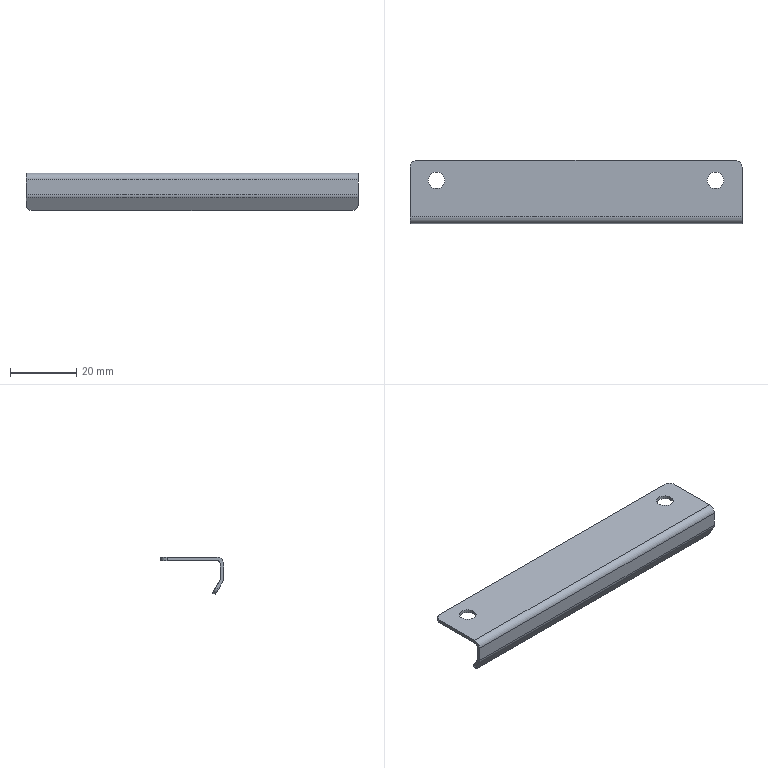Part | NX | features BREP 1 | 1 solid | 22 faces | box 100 x 19 x 11.33 mm | volume 2864 mm3 | cylinder 12 | plane 10 | commonest cylinder face diameters 4 x6 5 x4 2 x2
STEP:
#1=CARTESIAN_POINT('',(-39.5,3.5,1.));
#2=VERTEX_POINT('',#1);
#3=CARTESIAN_POINT('',(-44.5,3.5,1.));
#4=VERTEX_POINT('',#3);
#5=CARTESIAN_POINT('',(-42.,3.5,1.));
#6=DIRECTION('',(0.,0.,-1.));
#7=DIRECTION('',(-1.,0.,0.));
#8=AXIS2_PLACEMENT_3D('',#5,#6,#7);
#9=CIRCLE('',#8,2.5);
#10=EDGE_CURVE('',#2,#4,#9,.T.);
#11=ORIENTED_EDGE('',*,*,#10,.F.);
#12=CARTESIAN_POINT('',(-39.5,3.5,0.));
#13=VERTEX_POINT('',#12);
#14=CARTESIAN_POINT('',(-39.5,3.5,1.));
#15=DIRECTION('',(0.,0.,-1.));
#16=VECTOR('',#15,1000.);
#17=LINE('',#14,#16);
#18=EDGE_CURVE('',#2,#13,#17,.T.);
#19=ORIENTED_EDGE('',*,*,#18,.T.);
#20=CARTESIAN_POINT('',(-44.5,3.5,0.));
#21=VERTEX_POINT('',#20);
#22=CARTESIAN_POINT('',(-42.,3.5,0.));
#23=DIRECTION('',(0.,0.,-1.));
#24=DIRECTION('',(-1.,0.,0.));
#25=AXIS2_PLACEMENT_3D('',#22,#23,#24);
#26=CIRCLE('',#25,2.5);
#27=EDGE_CURVE('',#13,#21,#26,.T.);
#28=ORIENTED_EDGE('',*,*,#27,.T.);
#29=CARTESIAN_POINT('',(-44.5,3.5,1.));
#30=DIRECTION('',(0.,0.,-1.));
#31=VECTOR('',#30,1000.);
#32=LINE('',#29,#31);
#33=EDGE_CURVE('',#4,#21,#32,.T.);
#34=ORIENTED_EDGE('',*,*,#33,.F.);
#35=EDGE_LOOP('',(#11,#19,#28,#34));
#36=FACE_BOUND('',#35,.T.);
#37=CARTESIAN_POINT('',(-42.,3.5,1.));
#38=DIRECTION('',(0.,0.,-1.));
#39=DIRECTION('',(-1.,0.,0.));
#40=AXIS2_PLACEMENT_3D('',#37,#38,#39);
#41=CYLINDRICAL_SURFACE('',#40,2.5);
#42=ADVANCED_FACE('',(#36),#41,.F.);
#43=CARTESIAN_POINT('',(44.5,3.5,1.));
#44=VERTEX_POINT('',#43);
#45=CARTESIAN_POINT('',(39.5,3.5,1.));
#46=VERTEX_POINT('',#45);
#47=CARTESIAN_POINT('',(42.,3.5,1.));
#48=DIRECTION('',(0.,0.,-1.));
#49=DIRECTION('',(-1.,0.,0.));
#50=AXIS2_PLACEMENT_3D('',#47,#48,#49);
#51=CIRCLE('',#50,2.5);
#52=EDGE_CURVE('',#44,#46,#51,.T.);
#53=ORIENTED_EDGE('',*,*,#52,.F.);
#54=CARTESIAN_POINT('',(44.5,3.5,0.));
#55=VERTEX_POINT('',#54);
#56=CARTESIAN_POINT('',(44.5,3.5,1.));
#57=DIRECTION('',(0.,0.,-1.));
#58=VECTOR('',#57,1000.);
#59=LINE('',#56,#58);
#60=EDGE_CURVE('',#44,#55,#59,.T.);
#61=ORIENTED_EDGE('',*,*,#60,.T.);
#62=CARTESIAN_POINT('',(39.5,3.5,0.));
#63=VERTEX_POINT('',#62);
#64=CARTESIAN_POINT('',(42.,3.5,0.));
#65=DIRECTION('',(0.,0.,-1.));
#66=DIRECTION('',(-1.,0.,0.));
#67=AXIS2_PLACEMENT_3D('',#64,#65,#66);
#68=CIRCLE('',#67,2.5);
#69=EDGE_CURVE('',#55,#63,#68,.T.);
#70=ORIENTED_EDGE('',*,*,#69,.T.);
#71=CARTESIAN_POINT('',(39.5,3.5,1.));
#72=DIRECTION('',(0.,0.,-1.));
#73=VECTOR('',#72,1000.);
#74=LINE('',#71,#73);
#75=EDGE_CURVE('',#46,#63,#74,.T.);
#76=ORIENTED_EDGE('',*,*,#75,.F.);
#77=EDGE_LOOP('',(#53,#61,#70,#76));
#78=FACE_BOUND('',#77,.T.);
#79=CARTESIAN_POINT('',(42.,3.5,1.));
#80=DIRECTION('',(0.,0.,-1.));
#81=DIRECTION('',(-1.,0.,0.));
#82=AXIS2_PLACEMENT_3D('',#79,#80,#81);
#83=CYLINDRICAL_SURFACE('',#82,2.5);
#84=ADVANCED_FACE('',(#78),#83,.F.);
#85=CARTESIAN_POINT('',(50.,-9.232,-6.464));
#86=VERTEX_POINT('',#85);
#87=CARTESIAN_POINT('',(50.,-8.,-8.598));
#88=VERTEX_POINT('',#87);
#89=CARTESIAN_POINT('',(50.,-9.5,-6.));
#90=DIRECTION('',(0.,0.5,-0.866));
#91=VECTOR('',#90,1000.);
#92=LINE('',#89,#91);
#93=EDGE_CURVE('',#86,#88,#92,.T.);
#94=ORIENTED_EDGE('',*,*,#93,.T.);
#95=CARTESIAN_POINT('',(50.,-7.134,-8.098));
#96=VERTEX_POINT('',#95);
#97=CARTESIAN_POINT('',(50.,-7.134,-8.098));
#98=DIRECTION('',(0.,0.866,0.5));
#99=VECTOR('',#98,1000.);
#100=LINE('',#97,#99);
#101=EDGE_CURVE('',#88,#96,#100,.T.);
#102=ORIENTED_EDGE('',*,*,#101,.T.);
#103=CARTESIAN_POINT('',(50.,-8.366,-5.964));
#104=VERTEX_POINT('',#103);
#105=CARTESIAN_POINT('',(50.,-8.634,-5.5));
#106=DIRECTION('',(0.,-0.5,0.866));
#107=VECTOR('',#106,1000.);
#108=LINE('',#105,#107);
#109=EDGE_CURVE('',#96,#104,#108,.T.);
#110=ORIENTED_EDGE('',*,*,#109,.T.);
#111=CARTESIAN_POINT('',(50.,-8.5,-5.464));
#112=VERTEX_POINT('',#111);
#113=CARTESIAN_POINT('',(50.,-7.5,-5.464));
#114=DIRECTION('',(-1.,0.,0.));
#115=DIRECTION('',(0.,0.,1.));
#116=AXIS2_PLACEMENT_3D('',#113,#114,#115);
#117=CIRCLE('',#116,1.);
#118=EDGE_CURVE('',#104,#112,#117,.T.);
#119=ORIENTED_EDGE('',*,*,#118,.T.);
#120=CARTESIAN_POINT('',(50.,-8.5,-1.));
#121=VERTEX_POINT('',#120);
#122=CARTESIAN_POINT('',(50.,-8.5,-6.));
#123=DIRECTION('',(0.,0.,1.));
#124=VECTOR('',#123,1000.);
#125=LINE('',#122,#124);
#126=EDGE_CURVE('',#112,#121,#125,.T.);
#127=ORIENTED_EDGE('',*,*,#126,.T.);
#128=CARTESIAN_POINT('',(50.,-7.5,0.));
#129=VERTEX_POINT('',#128);
#130=CARTESIAN_POINT('',(50.,-7.5,-1.));
#131=DIRECTION('',(-1.,0.,0.));
#132=DIRECTION('',(0.,0.,1.));
#133=AXIS2_PLACEMENT_3D('',#130,#131,#132);
#134=CIRCLE('',#133,1.);
#135=EDGE_CURVE('',#121,#129,#134,.T.);
#136=ORIENTED_EDGE('',*,*,#135,.T.);
#137=CARTESIAN_POINT('',(50.,7.5,0.));
#138=VERTEX_POINT('',#137);
#139=CARTESIAN_POINT('',(50.,-9.5,0.));
#140=DIRECTION('',(0.,1.,0.));
#141=VECTOR('',#140,1000.);
#142=LINE('',#139,#141);
#143=EDGE_CURVE('',#129,#138,#142,.T.);
#144=ORIENTED_EDGE('',*,*,#143,.T.);
#145=CARTESIAN_POINT('',(50.,7.5,1.));
#146=VERTEX_POINT('',#145);
#147=CARTESIAN_POINT('',(50.,7.5,1.));
#148=DIRECTION('',(0.,0.,1.));
#149=VECTOR('',#148,1000.);
#150=LINE('',#147,#149);
#151=EDGE_CURVE('',#138,#146,#150,.T.);
#152=ORIENTED_EDGE('',*,*,#151,.T.);
#153=CARTESIAN_POINT('',(50.,-7.5,1.));
#154=VERTEX_POINT('',#153);
#155=CARTESIAN_POINT('',(50.,-9.5,1.));
#156=DIRECTION('',(0.,1.,0.));
#157=VECTOR('',#156,1000.);
#158=LINE('',#155,#157);
#159=EDGE_CURVE('',#154,#146,#158,.T.);
#160=ORIENTED_EDGE('',*,*,#159,.F.);
#161=CARTESIAN_POINT('',(50.,-9.5,-1.));
#162=VERTEX_POINT('',#161);
#163=CARTESIAN_POINT('',(50.,-7.5,-1.));
#164=DIRECTION('',(1.,0.,0.));
#165=DIRECTION('',(0.,0.,1.));
#166=AXIS2_PLACEMENT_3D('',#163,#164,#165);
#167=CIRCLE('',#166,2.);
#168=EDGE_CURVE('',#154,#162,#167,.T.);
#169=ORIENTED_EDGE('',*,*,#168,.T.);
#170=CARTESIAN_POINT('',(50.,-9.5,-5.464));
#171=VERTEX_POINT('',#170);
#172=CARTESIAN_POINT('',(50.,-9.5,1.));
#173=DIRECTION('',(0.,0.,-1.));
#174=VECTOR('',#173,1000.);
#175=LINE('',#172,#174);
#176=EDGE_CURVE('',#162,#171,#175,.T.);
#177=ORIENTED_EDGE('',*,*,#176,.T.);
#178=CARTESIAN_POINT('',(50.,-7.5,-5.464));
#179=DIRECTION('',(1.,0.,0.));
#180=DIRECTION('',(0.,0.,1.));
#181=AXIS2_PLACEMENT_3D('',#178,#179,#180);
#182=CIRCLE('',#181,2.);
#183=EDGE_CURVE('',#171,#86,#182,.T.);
#184=ORIENTED_EDGE('',*,*,#183,.T.);
#185=EDGE_LOOP('',(#94,#102,#110,#119,#127,#136,#144,#152,#160,#169,#177,#184));
#186=FACE_BOUND('',#185,.T.);
#187=CARTESIAN_POINT('',(50.,-9.5,1.));
#188=DIRECTION('',(-1.,0.,0.));
#189=DIRECTION('',(0.,0.,1.));
#190=AXIS2_PLACEMENT_3D('',#187,#188,#189);
#191=PLANE('',#190);
#192=ADVANCED_FACE('',(#186),#191,.F.);
#193=CARTESIAN_POINT('',(48.,9.5,1.));
#194=VERTEX_POINT('',#193);
#195=CARTESIAN_POINT('',(-48.,9.5,1.));
#196=VERTEX_POINT('',#195);
#197=CARTESIAN_POINT('',(-50.,9.5,1.));
#198=DIRECTION('',(-1.,0.,0.));
#199=VECTOR('',#198,1000.);
#200=LINE('',#197,#199);
#201=EDGE_CURVE('',#194,#196,#200,.T.);
#202=ORIENTED_EDGE('',*,*,#201,.F.);
#203=CARTESIAN_POINT('',(48.,9.5,0.));
#204=VERTEX_POINT('',#203);
#205=CARTESIAN_POINT('',(48.,9.5,1.));
#206=DIRECTION('',(0.,0.,-1.));
#207=VECTOR('',#206,1000.);
#208=LINE('',#205,#207);
#209=EDGE_CURVE('',#194,#204,#208,.T.);
#210=ORIENTED_EDGE('',*,*,#209,.T.);
#211=CARTESIAN_POINT('',(-48.,9.5,0.));
#212=VERTEX_POINT('',#211);
#213=CARTESIAN_POINT('',(-50.,9.5,0.));
#214=DIRECTION('',(-1.,0.,0.));
#215=VECTOR('',#214,1000.);
#216=LINE('',#213,#215);
#217=EDGE_CURVE('',#204,#212,#216,.T.);
#218=ORIENTED_EDGE('',*,*,#217,.T.);
#219=CARTESIAN_POINT('',(-48.,9.5,1.));
#220=DIRECTION('',(0.,0.,1.));
#221=VECTOR('',#220,1000.);
#222=LINE('',#219,#221);
#223=EDGE_CURVE('',#212,#196,#222,.T.);
#224=ORIENTED_EDGE('',*,*,#223,.T.);
#225=EDGE_LOOP('',(#202,#210,#218,#224));
#226=FACE_BOUND('',#225,.T.);
#227=CARTESIAN_POINT('',(-50.,9.5,1.));
#228=DIRECTION('',(0.,-1.,0.));
#229=DIRECTION('',(0.,0.,-1.));
#230=AXIS2_PLACEMENT_3D('',#227,#228,#229);
#231=PLANE('',#230);
#232=ADVANCED_FACE('',(#226),#231,.F.);
#233=CARTESIAN_POINT('',(-50.,-8.366,-5.964));
#234=VERTEX_POINT('',#233);
#235=CARTESIAN_POINT('',(-50.,-7.134,-8.098));
#236=VERTEX_POINT('',#235);
#237=CARTESIAN_POINT('',(-50.,-8.634,-5.5));
#238=DIRECTION('',(0.,0.5,-0.866));
#239=VECTOR('',#238,1000.);
#240=LINE('',#237,#239);
#241=EDGE_CURVE('',#234,#236,#240,.T.);
#242=ORIENTED_EDGE('',*,*,#241,.T.);
#243=CARTESIAN_POINT('',(-50.,-8.,-8.598));
#244=VERTEX_POINT('',#243);
#245=CARTESIAN_POINT('',(-50.,-8.,-8.598));
#246=DIRECTION('',(0.,-0.866,-0.5));
#247=VECTOR('',#246,1000.);
#248=LINE('',#245,#247);
#249=EDGE_CURVE('',#236,#244,#248,.T.);
#250=ORIENTED_EDGE('',*,*,#249,.T.);
#251=CARTESIAN_POINT('',(-50.,-9.232,-6.464));
#252=VERTEX_POINT('',#251);
#253=CARTESIAN_POINT('',(-50.,-9.5,-6.));
#254=DIRECTION('',(0.,-0.5,0.866));
#255=VECTOR('',#254,1000.);
#256=LINE('',#253,#255);
#257=EDGE_CURVE('',#244,#252,#256,.T.);
#258=ORIENTED_EDGE('',*,*,#257,.T.);
#259=CARTESIAN_POINT('',(-50.,-9.5,-5.464));
#260=VERTEX_POINT('',#259);
#261=CARTESIAN_POINT('',(-50.,-7.5,-5.464));
#262=DIRECTION('',(-1.,0.,0.));
#263=DIRECTION('',(0.,0.,-1.));
#264=AXIS2_PLACEMENT_3D('',#261,#262,#263);
#265=CIRCLE('',#264,2.);
#266=EDGE_CURVE('',#252,#260,#265,.T.);
#267=ORIENTED_EDGE('',*,*,#266,.T.);
#268=CARTESIAN_POINT('',(-50.,-9.5,-1.));
#269=VERTEX_POINT('',#268);
#270=CARTESIAN_POINT('',(-50.,-9.5,1.));
#271=DIRECTION('',(0.,0.,-1.));
#272=VECTOR('',#271,1000.);
#273=LINE('',#270,#272);
#274=EDGE_CURVE('',#269,#260,#273,.T.);
#275=ORIENTED_EDGE('',*,*,#274,.F.);
#276=CARTESIAN_POINT('',(-50.,-7.5,1.));
#277=VERTEX_POINT('',#276);
#278=CARTESIAN_POINT('',(-50.,-7.5,-1.));
#279=DIRECTION('',(-1.,0.,0.));
#280=DIRECTION('',(0.,0.,-1.));
#281=AXIS2_PLACEMENT_3D('',#278,#279,#280);
#282=CIRCLE('',#281,2.);
#283=EDGE_CURVE('',#269,#277,#282,.T.);
#284=ORIENTED_EDGE('',*,*,#283,.T.);
#285=CARTESIAN_POINT('',(-50.,7.5,1.));
#286=VERTEX_POINT('',#285);
#287=CARTESIAN_POINT('',(-50.,-9.5,1.));
#288=DIRECTION('',(0.,-1.,0.));
#289=VECTOR('',#288,1000.);
#290=LINE('',#287,#289);
#291=EDGE_CURVE('',#286,#277,#290,.T.);
#292=ORIENTED_EDGE('',*,*,#291,.F.);
#293=CARTESIAN_POINT('',(-50.,7.5,0.));
#294=VERTEX_POINT('',#293);
#295=CARTESIAN_POINT('',(-50.,7.5,1.));
#296=DIRECTION('',(0.,0.,-1.));
#297=VECTOR('',#296,1000.);
#298=LINE('',#295,#297);
#299=EDGE_CURVE('',#286,#294,#298,.T.);
#300=ORIENTED_EDGE('',*,*,#299,.T.);
#301=CARTESIAN_POINT('',(-50.,-7.5,0.));
#302=VERTEX_POINT('',#301);
#303=CARTESIAN_POINT('',(-50.,-9.5,0.));
#304=DIRECTION('',(0.,-1.,0.));
#305=VECTOR('',#304,1000.);
#306=LINE('',#303,#305);
#307=EDGE_CURVE('',#294,#302,#306,.T.);
#308=ORIENTED_EDGE('',*,*,#307,.T.);
#309=CARTESIAN_POINT('',(-50.,-8.5,-1.));
#310=VERTEX_POINT('',#309);
#311=CARTESIAN_POINT('',(-50.,-7.5,-1.));
#312=DIRECTION('',(1.,0.,0.));
#313=DIRECTION('',(0.,0.,-1.));
#314=AXIS2_PLACEMENT_3D('',#311,#312,#313);
#315=CIRCLE('',#314,1.);
#316=EDGE_CURVE('',#302,#310,#315,.T.);
#317=ORIENTED_EDGE('',*,*,#316,.T.);
#318=CARTESIAN_POINT('',(-50.,-8.5,-5.464));
#319=VERTEX_POINT('',#318);
#320=CARTESIAN_POINT('',(-50.,-8.5,-6.));
#321=DIRECTION('',(0.,0.,1.));
#322=VECTOR('',#321,1000.);
#323=LINE('',#320,#322);
#324=EDGE_CURVE('',#319,#310,#323,.T.);
#325=ORIENTED_EDGE('',*,*,#324,.F.);
#326=CARTESIAN_POINT('',(-50.,-7.5,-5.464));
#327=DIRECTION('',(1.,0.,0.));
#328=DIRECTION('',(0.,0.,-1.));
#329=AXIS2_PLACEMENT_3D('',#326,#327,#328);
#330=CIRCLE('',#329,1.);
#331=EDGE_CURVE('',#319,#234,#330,.T.);
#332=ORIENTED_EDGE('',*,*,#331,.T.);
#333=EDGE_LOOP('',(#242,#250,#258,#267,#275,#284,#292,#300,#308,#317,#325,#332));
#334=FACE_BOUND('',#333,.T.);
#335=CARTESIAN_POINT('',(-50.,-9.5,1.));
#336=DIRECTION('',(1.,0.,0.));
#337=DIRECTION('',(0.,1.,0.));
#338=AXIS2_PLACEMENT_3D('',#335,#336,#337);
#339=PLANE('',#338);
#340=ADVANCED_FACE('',(#334),#339,.F.);
#341=ORIENTED_EDGE('',*,*,#274,.T.);
#342=CARTESIAN_POINT('',(50.,-9.5,-5.464));
#343=DIRECTION('',(1.,0.,0.));
#344=VECTOR('',#343,1000.);
#345=LINE('',#342,#344);
#346=EDGE_CURVE('',#260,#171,#345,.T.);
#347=ORIENTED_EDGE('',*,*,#346,.T.);
#348=ORIENTED_EDGE('',*,*,#176,.F.);
#349=CARTESIAN_POINT('',(-50.,-9.5,-1.));
#350=DIRECTION('',(-1.,0.,0.));
#351=VECTOR('',#350,1000.);
#352=LINE('',#349,#351);
#353=EDGE_CURVE('',#162,#269,#352,.T.);
#354=ORIENTED_EDGE('',*,*,#353,.T.);
#355=EDGE_LOOP('',(#341,#347,#348,#354));
#356=FACE_BOUND('',#355,.T.);
#357=CARTESIAN_POINT('',(-50.,-9.5,1.));
#358=DIRECTION('',(0.,1.,0.));
#359=DIRECTION('',(1.,0.,0.));
#360=AXIS2_PLACEMENT_3D('',#357,#358,#359);
#361=PLANE('',#360);
#362=ADVANCED_FACE('',(#356),#361,.F.);
#363=ORIENTED_EDGE('',*,*,#159,.T.);
#364=CARTESIAN_POINT('',(48.,7.5,1.));
#365=DIRECTION('',(0.,0.,1.));
#366=DIRECTION('',(-1.,0.,0.));
#367=AXIS2_PLACEMENT_3D('',#364,#365,#366);
#368=CIRCLE('',#367,2.);
#369=EDGE_CURVE('',#146,#194,#368,.T.);
#370=ORIENTED_EDGE('',*,*,#369,.T.);
#371=ORIENTED_EDGE('',*,*,#201,.T.);
#372=CARTESIAN_POINT('',(-48.,7.5,1.));
#373=DIRECTION('',(0.,0.,1.));
#374=DIRECTION('',(-1.,0.,0.));
#375=AXIS2_PLACEMENT_3D('',#372,#373,#374);
#376=CIRCLE('',#375,2.);
#377=EDGE_CURVE('',#196,#286,#376,.T.);
#378=ORIENTED_EDGE('',*,*,#377,.T.);
#379=ORIENTED_EDGE('',*,*,#291,.T.);
#380=CARTESIAN_POINT('',(0.,-7.5,1.));
#381=DIRECTION('',(1.,0.,0.));
#382=VECTOR('',#381,1000.);
#383=LINE('',#380,#382);
#384=EDGE_CURVE('',#277,#154,#383,.T.);
#385=ORIENTED_EDGE('',*,*,#384,.T.);
#386=EDGE_LOOP('',(#363,#370,#371,#378,#379,#385));
#387=FACE_BOUND('',#386,.T.);
#388=CARTESIAN_POINT('',(-42.,3.5,1.));
#389=DIRECTION('',(0.,0.,-1.));
#390=DIRECTION('',(-1.,0.,0.));
#391=AXIS2_PLACEMENT_3D('',#388,#389,#390);
#392=CIRCLE('',#391,2.5);
#393=EDGE_CURVE('',#4,#2,#392,.T.);
#394=ORIENTED_EDGE('',*,*,#393,.T.);
#395=ORIENTED_EDGE('',*,*,#10,.T.);
#396=EDGE_LOOP('',(#394,#395));
#397=FACE_BOUND('',#396,.T.);
#398=CARTESIAN_POINT('',(42.,3.5,1.));
#399=DIRECTION('',(0.,0.,-1.));
#400=DIRECTION('',(-1.,0.,0.));
#401=AXIS2_PLACEMENT_3D('',#398,#399,#400);
#402=CIRCLE('',#401,2.5);
#403=EDGE_CURVE('',#46,#44,#402,.T.);
#404=ORIENTED_EDGE('',*,*,#403,.T.);
#405=ORIENTED_EDGE('',*,*,#52,.T.);
#406=EDGE_LOOP('',(#404,#405));
#407=FACE_BOUND('',#406,.T.);
#408=CARTESIAN_POINT('',(0.,0.,1.));
#409=DIRECTION('',(0.,0.,-1.));
#410=DIRECTION('',(0.,-1.,0.));
#411=AXIS2_PLACEMENT_3D('',#408,#409,#410);
#412=PLANE('',#411);
#413=ADVANCED_FACE('',(#387,#397,#407),#412,.F.);
#414=ORIENTED_EDGE('',*,*,#217,.F.);
#415=CARTESIAN_POINT('',(48.,7.5,0.));
#416=DIRECTION('',(0.,0.,-1.));
#417=DIRECTION('',(-1.,0.,0.));
#418=AXIS2_PLACEMENT_3D('',#415,#416,#417);
#419=CIRCLE('',#418,2.);
#420=EDGE_CURVE('',#204,#138,#419,.T.);
#421=ORIENTED_EDGE('',*,*,#420,.T.);
#422=ORIENTED_EDGE('',*,*,#143,.F.);
#423=CARTESIAN_POINT('',(0.,-7.5,0.));
#424=DIRECTION('',(-1.,0.,0.));
#425=VECTOR('',#424,1000.);
#426=LINE('',#423,#425);
#427=EDGE_CURVE('',#129,#302,#426,.T.);
#428=ORIENTED_EDGE('',*,*,#427,.T.);
#429=ORIENTED_EDGE('',*,*,#307,.F.);
#430=CARTESIAN_POINT('',(-48.,7.5,0.));
#431=DIRECTION('',(0.,0.,-1.));
#432=DIRECTION('',(-1.,0.,0.));
#433=AXIS2_PLACEMENT_3D('',#430,#431,#432);
#434=CIRCLE('',#433,2.);
#435=EDGE_CURVE('',#294,#212,#434,.T.);
#436=ORIENTED_EDGE('',*,*,#435,.T.);
#437=EDGE_LOOP('',(#414,#421,#422,#428,#429,#436));
#438=FACE_BOUND('',#437,.T.);
#439=CARTESIAN_POINT('',(-42.,3.5,0.));
#440=DIRECTION('',(0.,0.,-1.));
#441=DIRECTION('',(-1.,0.,0.));
#442=AXIS2_PLACEMENT_3D('',#439,#440,#441);
#443=CIRCLE('',#442,2.5);
#444=EDGE_CURVE('',#21,#13,#443,.T.);
#445=ORIENTED_EDGE('',*,*,#444,.F.);
#446=ORIENTED_EDGE('',*,*,#27,.F.);
#447=EDGE_LOOP('',(#445,#446));
#448=FACE_BOUND('',#447,.T.);
#449=CARTESIAN_POINT('',(42.,3.5,0.));
#450=DIRECTION('',(0.,0.,-1.));
#451=DIRECTION('',(-1.,0.,0.));
#452=AXIS2_PLACEMENT_3D('',#449,#450,#451);
#453=CIRCLE('',#452,2.5);
#454=EDGE_CURVE('',#63,#55,#453,.T.);
#455=ORIENTED_EDGE('',*,*,#454,.F.);
#456=ORIENTED_EDGE('',*,*,#69,.F.);
#457=EDGE_LOOP('',(#455,#456));
#458=FACE_BOUND('',#457,.T.);
#459=CARTESIAN_POINT('',(0.,0.,0.));
#460=DIRECTION('',(0.,0.,-1.));
#461=DIRECTION('',(0.,-1.,0.));
#462=AXIS2_PLACEMENT_3D('',#459,#460,#461);
#463=PLANE('',#462);
#464=ADVANCED_FACE('',(#438,#448,#458),#463,.T.);
#465=ORIENTED_EDGE('',*,*,#126,.F.);
#466=CARTESIAN_POINT('',(-50.,-8.5,-5.464));
#467=DIRECTION('',(-1.,0.,0.));
#468=VECTOR('',#467,1000.);
#469=LINE('',#466,#468);
#470=EDGE_CURVE('',#112,#319,#469,.T.);
#471=ORIENTED_EDGE('',*,*,#470,.T.);
#472=ORIENTED_EDGE('',*,*,#324,.T.);
#473=CARTESIAN_POINT('',(-50.,-8.5,-1.));
#474=DIRECTION('',(1.,0.,0.));
#475=VECTOR('',#474,1000.);
#476=LINE('',#473,#475);
#477=EDGE_CURVE('',#310,#121,#476,.T.);
#478=ORIENTED_EDGE('',*,*,#477,.T.);
#479=EDGE_LOOP('',(#465,#471,#472,#478));
#480=FACE_BOUND('',#479,.T.);
#481=CARTESIAN_POINT('',(-50.,-8.5,-6.));
#482=DIRECTION('',(0.,-1.,0.));
#483=DIRECTION('',(-1.,0.,0.));
#484=AXIS2_PLACEMENT_3D('',#481,#482,#483);
#485=PLANE('',#484);
#486=ADVANCED_FACE('',(#480),#485,.F.);
#487=CARTESIAN_POINT('',(48.,-6.134,-9.83));
#488=VERTEX_POINT('',#487);
#489=CARTESIAN_POINT('',(-48.,-6.134,-9.83));
#490=VERTEX_POINT('',#489);
#491=CARTESIAN_POINT('',(55.887,-6.134,-9.83));
#492=DIRECTION('',(-1.,0.,0.));
#493=VECTOR('',#492,1000.);
#494=LINE('',#491,#493);
#495=EDGE_CURVE('',#488,#490,#494,.T.);
#496=ORIENTED_EDGE('',*,*,#495,.T.);
#497=CARTESIAN_POINT('',(-48.,-7.134,-8.098));
#498=DIRECTION('',(0.,0.866,0.5));
#499=DIRECTION('',(0.,-0.5,0.866));
#500=AXIS2_PLACEMENT_3D('',#497,#498,#499);
#501=CIRCLE('',#500,2.);
#502=EDGE_CURVE('',#490,#236,#501,.T.);
#503=ORIENTED_EDGE('',*,*,#502,.T.);
#504=ORIENTED_EDGE('',*,*,#241,.F.);
#505=CARTESIAN_POINT('',(55.887,-8.366,-5.964));
#506=DIRECTION('',(1.,0.,0.));
#507=VECTOR('',#506,1000.);
#508=LINE('',#505,#507);
#509=EDGE_CURVE('',#234,#104,#508,.T.);
#510=ORIENTED_EDGE('',*,*,#509,.T.);
#511=ORIENTED_EDGE('',*,*,#109,.F.);
#512=CARTESIAN_POINT('',(48.,-7.134,-8.098));
#513=DIRECTION('',(0.,0.866,0.5));
#514=DIRECTION('',(0.,-0.5,0.866));
#515=AXIS2_PLACEMENT_3D('',#512,#513,#514);
#516=CIRCLE('',#515,2.);
#517=EDGE_CURVE('',#96,#488,#516,.T.);
#518=ORIENTED_EDGE('',*,*,#517,.T.);
#519=EDGE_LOOP('',(#496,#503,#504,#510,#511,#518));
#520=FACE_BOUND('',#519,.T.);
#521=CARTESIAN_POINT('',(55.887,-8.634,-5.5));
#522=DIRECTION('',(0.,0.866,0.5));
#523=DIRECTION('',(1.,0.,0.));
#524=AXIS2_PLACEMENT_3D('',#521,#522,#523);
#525=PLANE('',#524);
#526=ADVANCED_FACE('',(#520),#525,.T.);
#527=ORIENTED_EDGE('',*,*,#257,.F.);
#528=CARTESIAN_POINT('',(-48.,-7.,-10.33));
#529=VERTEX_POINT('',#528);
#530=CARTESIAN_POINT('',(-48.,-8.,-8.598));
#531=DIRECTION('',(0.,-0.866,-0.5));
#532=DIRECTION('',(0.,0.5,-0.866));
#533=AXIS2_PLACEMENT_3D('',#530,#531,#532);
#534=CIRCLE('',#533,2.);
#535=EDGE_CURVE('',#244,#529,#534,.T.);
#536=ORIENTED_EDGE('',*,*,#535,.T.);
#537=CARTESIAN_POINT('',(48.,-7.,-10.33));
#538=VERTEX_POINT('',#537);
#539=CARTESIAN_POINT('',(55.887,-7.,-10.33));
#540=DIRECTION('',(-1.,0.,0.));
#541=VECTOR('',#540,1000.);
#542=LINE('',#539,#541);
#543=EDGE_CURVE('',#538,#529,#542,.T.);
#544=ORIENTED_EDGE('',*,*,#543,.F.);
#545=CARTESIAN_POINT('',(48.,-8.,-8.598));
#546=DIRECTION('',(0.,-0.866,-0.5));
#547=DIRECTION('',(0.,0.5,-0.866));
#548=AXIS2_PLACEMENT_3D('',#545,#546,#547);
#549=CIRCLE('',#548,2.);
#550=EDGE_CURVE('',#538,#88,#549,.T.);
#551=ORIENTED_EDGE('',*,*,#550,.T.);
#552=ORIENTED_EDGE('',*,*,#93,.F.);
#553=CARTESIAN_POINT('',(-50.,-9.232,-6.464));
#554=DIRECTION('',(-1.,0.,0.));
#555=VECTOR('',#554,1000.);
#556=LINE('',#553,#555);
#557=EDGE_CURVE('',#86,#252,#556,.T.);
#558=ORIENTED_EDGE('',*,*,#557,.T.);
#559=EDGE_LOOP('',(#527,#536,#544,#551,#552,#558));
#560=FACE_BOUND('',#559,.T.);
#561=CARTESIAN_POINT('',(55.887,-9.5,-6.));
#562=DIRECTION('',(0.,-0.866,-0.5));
#563=DIRECTION('',(0.,0.5,-0.866));
#564=AXIS2_PLACEMENT_3D('',#561,#562,#563);
#565=PLANE('',#564);
#566=ADVANCED_FACE('',(#560),#565,.T.);
#567=ORIENTED_EDGE('',*,*,#543,.T.);
#568=CARTESIAN_POINT('',(-48.,-6.134,-9.83));
#569=DIRECTION('',(0.,0.866,0.5));
#570=VECTOR('',#569,1000.);
#571=LINE('',#568,#570);
#572=EDGE_CURVE('',#529,#490,#571,.T.);
#573=ORIENTED_EDGE('',*,*,#572,.T.);
#574=ORIENTED_EDGE('',*,*,#495,.F.);
#575=CARTESIAN_POINT('',(48.,-7.,-10.33));
#576=DIRECTION('',(0.,-0.866,-0.5));
#577=VECTOR('',#576,1000.);
#578=LINE('',#575,#577);
#579=EDGE_CURVE('',#488,#538,#578,.T.);
#580=ORIENTED_EDGE('',*,*,#579,.T.);
#581=EDGE_LOOP('',(#567,#573,#574,#580));
#582=FACE_BOUND('',#581,.T.);
#583=CARTESIAN_POINT('',(55.887,-6.134,-9.83));
#584=DIRECTION('',(0.,0.5,-0.866));
#585=DIRECTION('',(-1.,0.,0.));
#586=AXIS2_PLACEMENT_3D('',#583,#584,#585);
#587=PLANE('',#586);
#588=ADVANCED_FACE('',(#582),#587,.T.);
#589=ORIENTED_EDGE('',*,*,#118,.F.);
#590=ORIENTED_EDGE('',*,*,#509,.F.);
#591=ORIENTED_EDGE('',*,*,#331,.F.);
#592=ORIENTED_EDGE('',*,*,#470,.F.);
#593=EDGE_LOOP('',(#589,#590,#591,#592));
#594=FACE_BOUND('',#593,.T.);
#595=CARTESIAN_POINT('',(-50.,-7.5,-5.464));
#596=DIRECTION('',(-1.,0.,0.));
#597=DIRECTION('',(0.,0.,1.));
#598=AXIS2_PLACEMENT_3D('',#595,#596,#597);
#599=CYLINDRICAL_SURFACE('',#598,1.);
#600=ADVANCED_FACE('',(#594),#599,.F.);
#601=ORIENTED_EDGE('',*,*,#316,.F.);
#602=ORIENTED_EDGE('',*,*,#427,.F.);
#603=ORIENTED_EDGE('',*,*,#135,.F.);
#604=ORIENTED_EDGE('',*,*,#477,.F.);
#605=EDGE_LOOP('',(#601,#602,#603,#604));
#606=FACE_BOUND('',#605,.T.);
#607=CARTESIAN_POINT('',(-50.,-7.5,-1.));
#608=DIRECTION('',(1.,0.,0.));
#609=DIRECTION('',(0.,1.,0.));
#610=AXIS2_PLACEMENT_3D('',#607,#608,#609);
#611=CYLINDRICAL_SURFACE('',#610,1.);
#612=ADVANCED_FACE('',(#606),#611,.F.);
#613=ORIENTED_EDGE('',*,*,#369,.F.);
#614=ORIENTED_EDGE('',*,*,#151,.F.);
#615=ORIENTED_EDGE('',*,*,#420,.F.);
#616=ORIENTED_EDGE('',*,*,#209,.F.);
#617=EDGE_LOOP('',(#613,#614,#615,#616));
#618=FACE_BOUND('',#617,.T.);
#619=CARTESIAN_POINT('',(48.,7.5,1.));
#620=DIRECTION('',(0.,0.,-1.));
#621=DIRECTION('',(-1.,0.,0.));
#622=AXIS2_PLACEMENT_3D('',#619,#620,#621);
#623=CYLINDRICAL_SURFACE('',#622,2.);
#624=ADVANCED_FACE('',(#618),#623,.T.);
#625=ORIENTED_EDGE('',*,*,#377,.F.);
#626=ORIENTED_EDGE('',*,*,#223,.F.);
#627=ORIENTED_EDGE('',*,*,#435,.F.);
#628=ORIENTED_EDGE('',*,*,#299,.F.);
#629=EDGE_LOOP('',(#625,#626,#627,#628));
#630=FACE_BOUND('',#629,.T.);
#631=CARTESIAN_POINT('',(-48.,7.5,1.));
#632=DIRECTION('',(0.,0.,-1.));
#633=DIRECTION('',(-1.,0.,0.));
#634=AXIS2_PLACEMENT_3D('',#631,#632,#633);
#635=CYLINDRICAL_SURFACE('',#634,2.);
#636=ADVANCED_FACE('',(#630),#635,.T.);
#637=ORIENTED_EDGE('',*,*,#183,.F.);
#638=ORIENTED_EDGE('',*,*,#346,.F.);
#639=ORIENTED_EDGE('',*,*,#266,.F.);
#640=ORIENTED_EDGE('',*,*,#557,.F.);
#641=EDGE_LOOP('',(#637,#638,#639,#640));
#642=FACE_BOUND('',#641,.T.);
#643=CARTESIAN_POINT('',(55.887,-7.5,-5.464));
#644=DIRECTION('',(1.,0.,0.));
#645=DIRECTION('',(0.,0.,-1.));
#646=AXIS2_PLACEMENT_3D('',#643,#644,#645);
#647=CYLINDRICAL_SURFACE('',#646,2.);
#648=ADVANCED_FACE('',(#642),#647,.T.);
#649=ORIENTED_EDGE('',*,*,#283,.F.);
#650=ORIENTED_EDGE('',*,*,#353,.F.);
#651=ORIENTED_EDGE('',*,*,#168,.F.);
#652=ORIENTED_EDGE('',*,*,#384,.F.);
#653=EDGE_LOOP('',(#649,#650,#651,#652));
#654=FACE_BOUND('',#653,.T.);
#655=CARTESIAN_POINT('',(0.,-7.5,-1.));
#656=DIRECTION('',(1.,0.,0.));
#657=DIRECTION('',(0.,0.,-1.));
#658=AXIS2_PLACEMENT_3D('',#655,#656,#657);
#659=CYLINDRICAL_SURFACE('',#658,2.);
#660=ADVANCED_FACE('',(#654),#659,.T.);
#661=ORIENTED_EDGE('',*,*,#60,.F.);
#662=ORIENTED_EDGE('',*,*,#403,.F.);
#663=ORIENTED_EDGE('',*,*,#75,.T.);
#664=ORIENTED_EDGE('',*,*,#454,.T.);
#665=EDGE_LOOP('',(#661,#662,#663,#664));
#666=FACE_BOUND('',#665,.T.);
#667=CARTESIAN_POINT('',(42.,3.5,1.));
#668=DIRECTION('',(0.,0.,-1.));
#669=DIRECTION('',(-1.,0.,0.));
#670=AXIS2_PLACEMENT_3D('',#667,#668,#669);
#671=CYLINDRICAL_SURFACE('',#670,2.5);
#672=ADVANCED_FACE('',(#666),#671,.F.);
#673=ORIENTED_EDGE('',*,*,#18,.F.);
#674=ORIENTED_EDGE('',*,*,#393,.F.);
#675=ORIENTED_EDGE('',*,*,#33,.T.);
#676=ORIENTED_EDGE('',*,*,#444,.T.);
#677=EDGE_LOOP('',(#673,#674,#675,#676));
#678=FACE_BOUND('',#677,.T.);
#679=CARTESIAN_POINT('',(-42.,3.5,1.));
#680=DIRECTION('',(0.,0.,-1.));
#681=DIRECTION('',(-1.,0.,0.));
#682=AXIS2_PLACEMENT_3D('',#679,#680,#681);
#683=CYLINDRICAL_SURFACE('',#682,2.5);
#684=ADVANCED_FACE('',(#678),#683,.F.);
#685=ORIENTED_EDGE('',*,*,#502,.F.);
#686=ORIENTED_EDGE('',*,*,#572,.F.);
#687=ORIENTED_EDGE('',*,*,#535,.F.);
#688=ORIENTED_EDGE('',*,*,#249,.F.);
#689=EDGE_LOOP('',(#685,#686,#687,#688));
#690=FACE_BOUND('',#689,.T.);
#691=CARTESIAN_POINT('',(-48.,-4.969,-6.848));
#692=DIRECTION('',(0.,0.866,0.5));
#693=DIRECTION('',(0.,-0.5,0.866));
#694=AXIS2_PLACEMENT_3D('',#691,#692,#693);
#695=CYLINDRICAL_SURFACE('',#694,2.);
#696=ADVANCED_FACE('',(#690),#695,.T.);
#697=ORIENTED_EDGE('',*,*,#550,.F.);
#698=ORIENTED_EDGE('',*,*,#579,.F.);
#699=ORIENTED_EDGE('',*,*,#517,.F.);
#700=ORIENTED_EDGE('',*,*,#101,.F.);
#701=EDGE_LOOP('',(#697,#698,#699,#700));
#702=FACE_BOUND('',#701,.T.);
#703=CARTESIAN_POINT('',(48.,-4.969,-6.848));
#704=DIRECTION('',(0.,-0.866,-0.5));
#705=DIRECTION('',(0.,0.5,-0.866));
#706=AXIS2_PLACEMENT_3D('',#703,#704,#705);
#707=CYLINDRICAL_SURFACE('',#706,2.);
#708=ADVANCED_FACE('',(#702),#707,.T.);
#709=CLOSED_SHELL('',(#42,#84,#192,#232,#340,#362,#413,#464,#486,#526,#566,#588,#600,#612,#624,#636,#648,#660,#672,#684,#696,#708));
#710=MANIFOLD_SOLID_BREP('',#709);
#711=(LENGTH_UNIT()NAMED_UNIT(*)SI_UNIT(.MILLI.,.METRE.));
#712=UNCERTAINTY_MEASURE_WITH_UNIT(LENGTH_MEASURE(0.00001),#711,'','');
#713=(NAMED_UNIT(*)PLANE_ANGLE_UNIT()SI_UNIT($,.RADIAN.));
#714=(NAMED_UNIT(*)SI_UNIT($,.STERADIAN.)SOLID_ANGLE_UNIT());
#715=(GEOMETRIC_REPRESENTATION_CONTEXT(3)GLOBAL_UNCERTAINTY_ASSIGNED_CONTEXT((#712))GLOBAL_UNIT_ASSIGNED_CONTEXT((#711,#713,#714))REPRESENTATION_CONTEXT('',''));
#716=ADVANCED_BREP_SHAPE_REPRESENTATION('',(#710),#715);